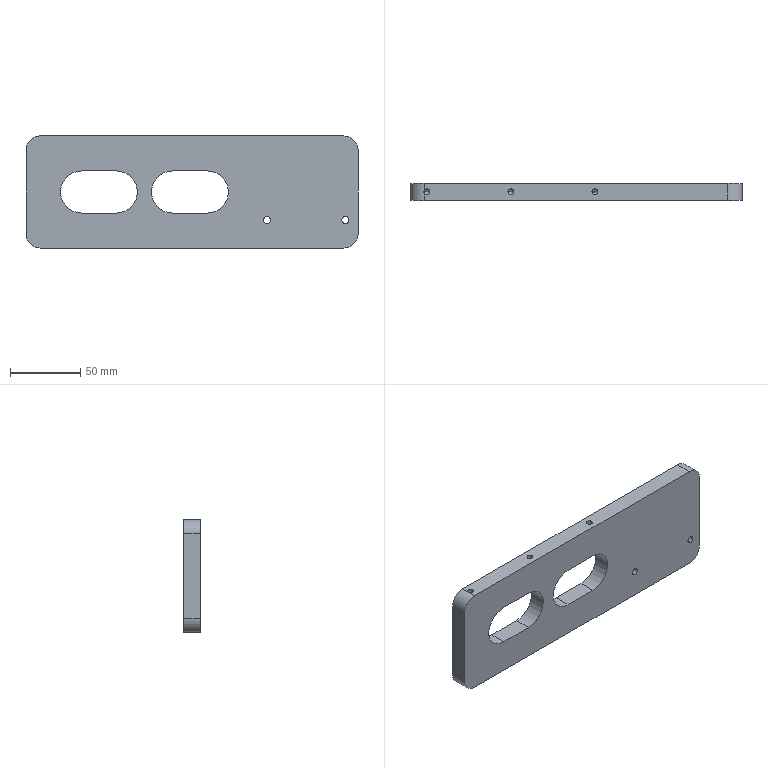Part | STEP file | support plate 6A_SUS304 | 1 solid | 34 faces | box 237 x 12 x 80 mm | volume 190372 mm3 | cylinder 18 | plane 10 | cone 6 | commonest cylinder face diameters 4.2 x6 5 x4 20 x4 30 x4